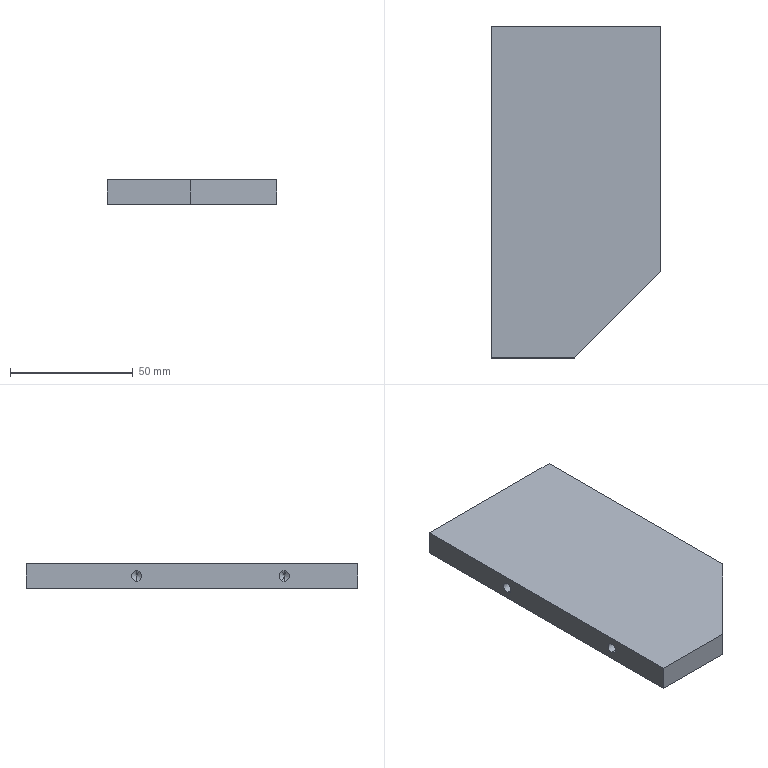Part | STEP file | 0244_215_Rib | 1 solid | 23 faces | box 69 x 135 x 10 mm | volume 86315 mm3 | cylinder 8 | cone 8 | plane 7 | commonest cylinder face diameters 4.2 x8